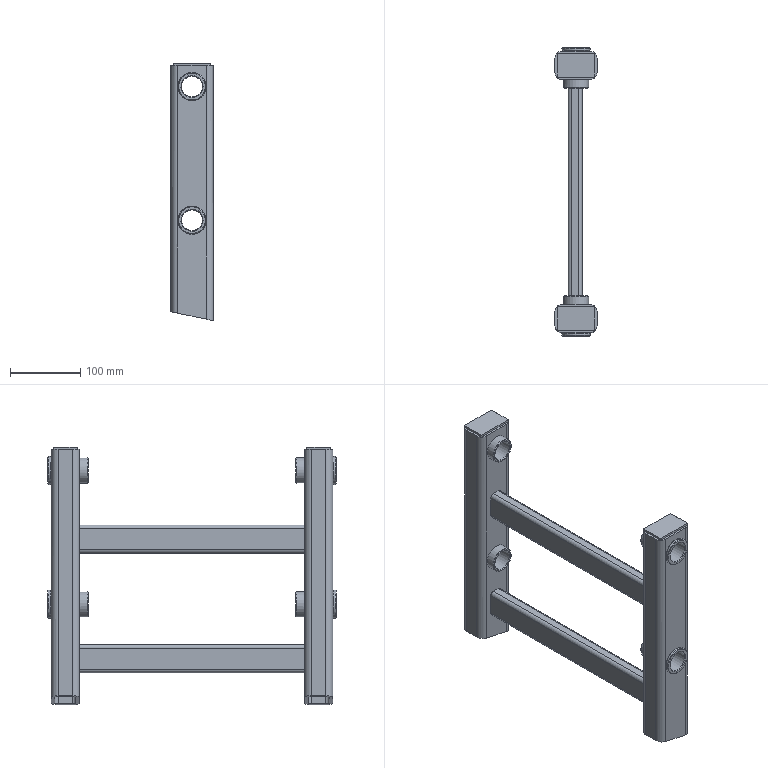Part | STEP file | HL4GZ-1.862.054 (gearbox mounting bracket weldment) | 10 solids | 136 faces | box 60 x 410 x 365.753 mm | volume 811040 mm3 | plane 64 | cylinder 52 | cone 20 | commonest cylinder face diameters 10 x16 5 x8 20 x8 36.5 x8 29.5 x4 36 x4